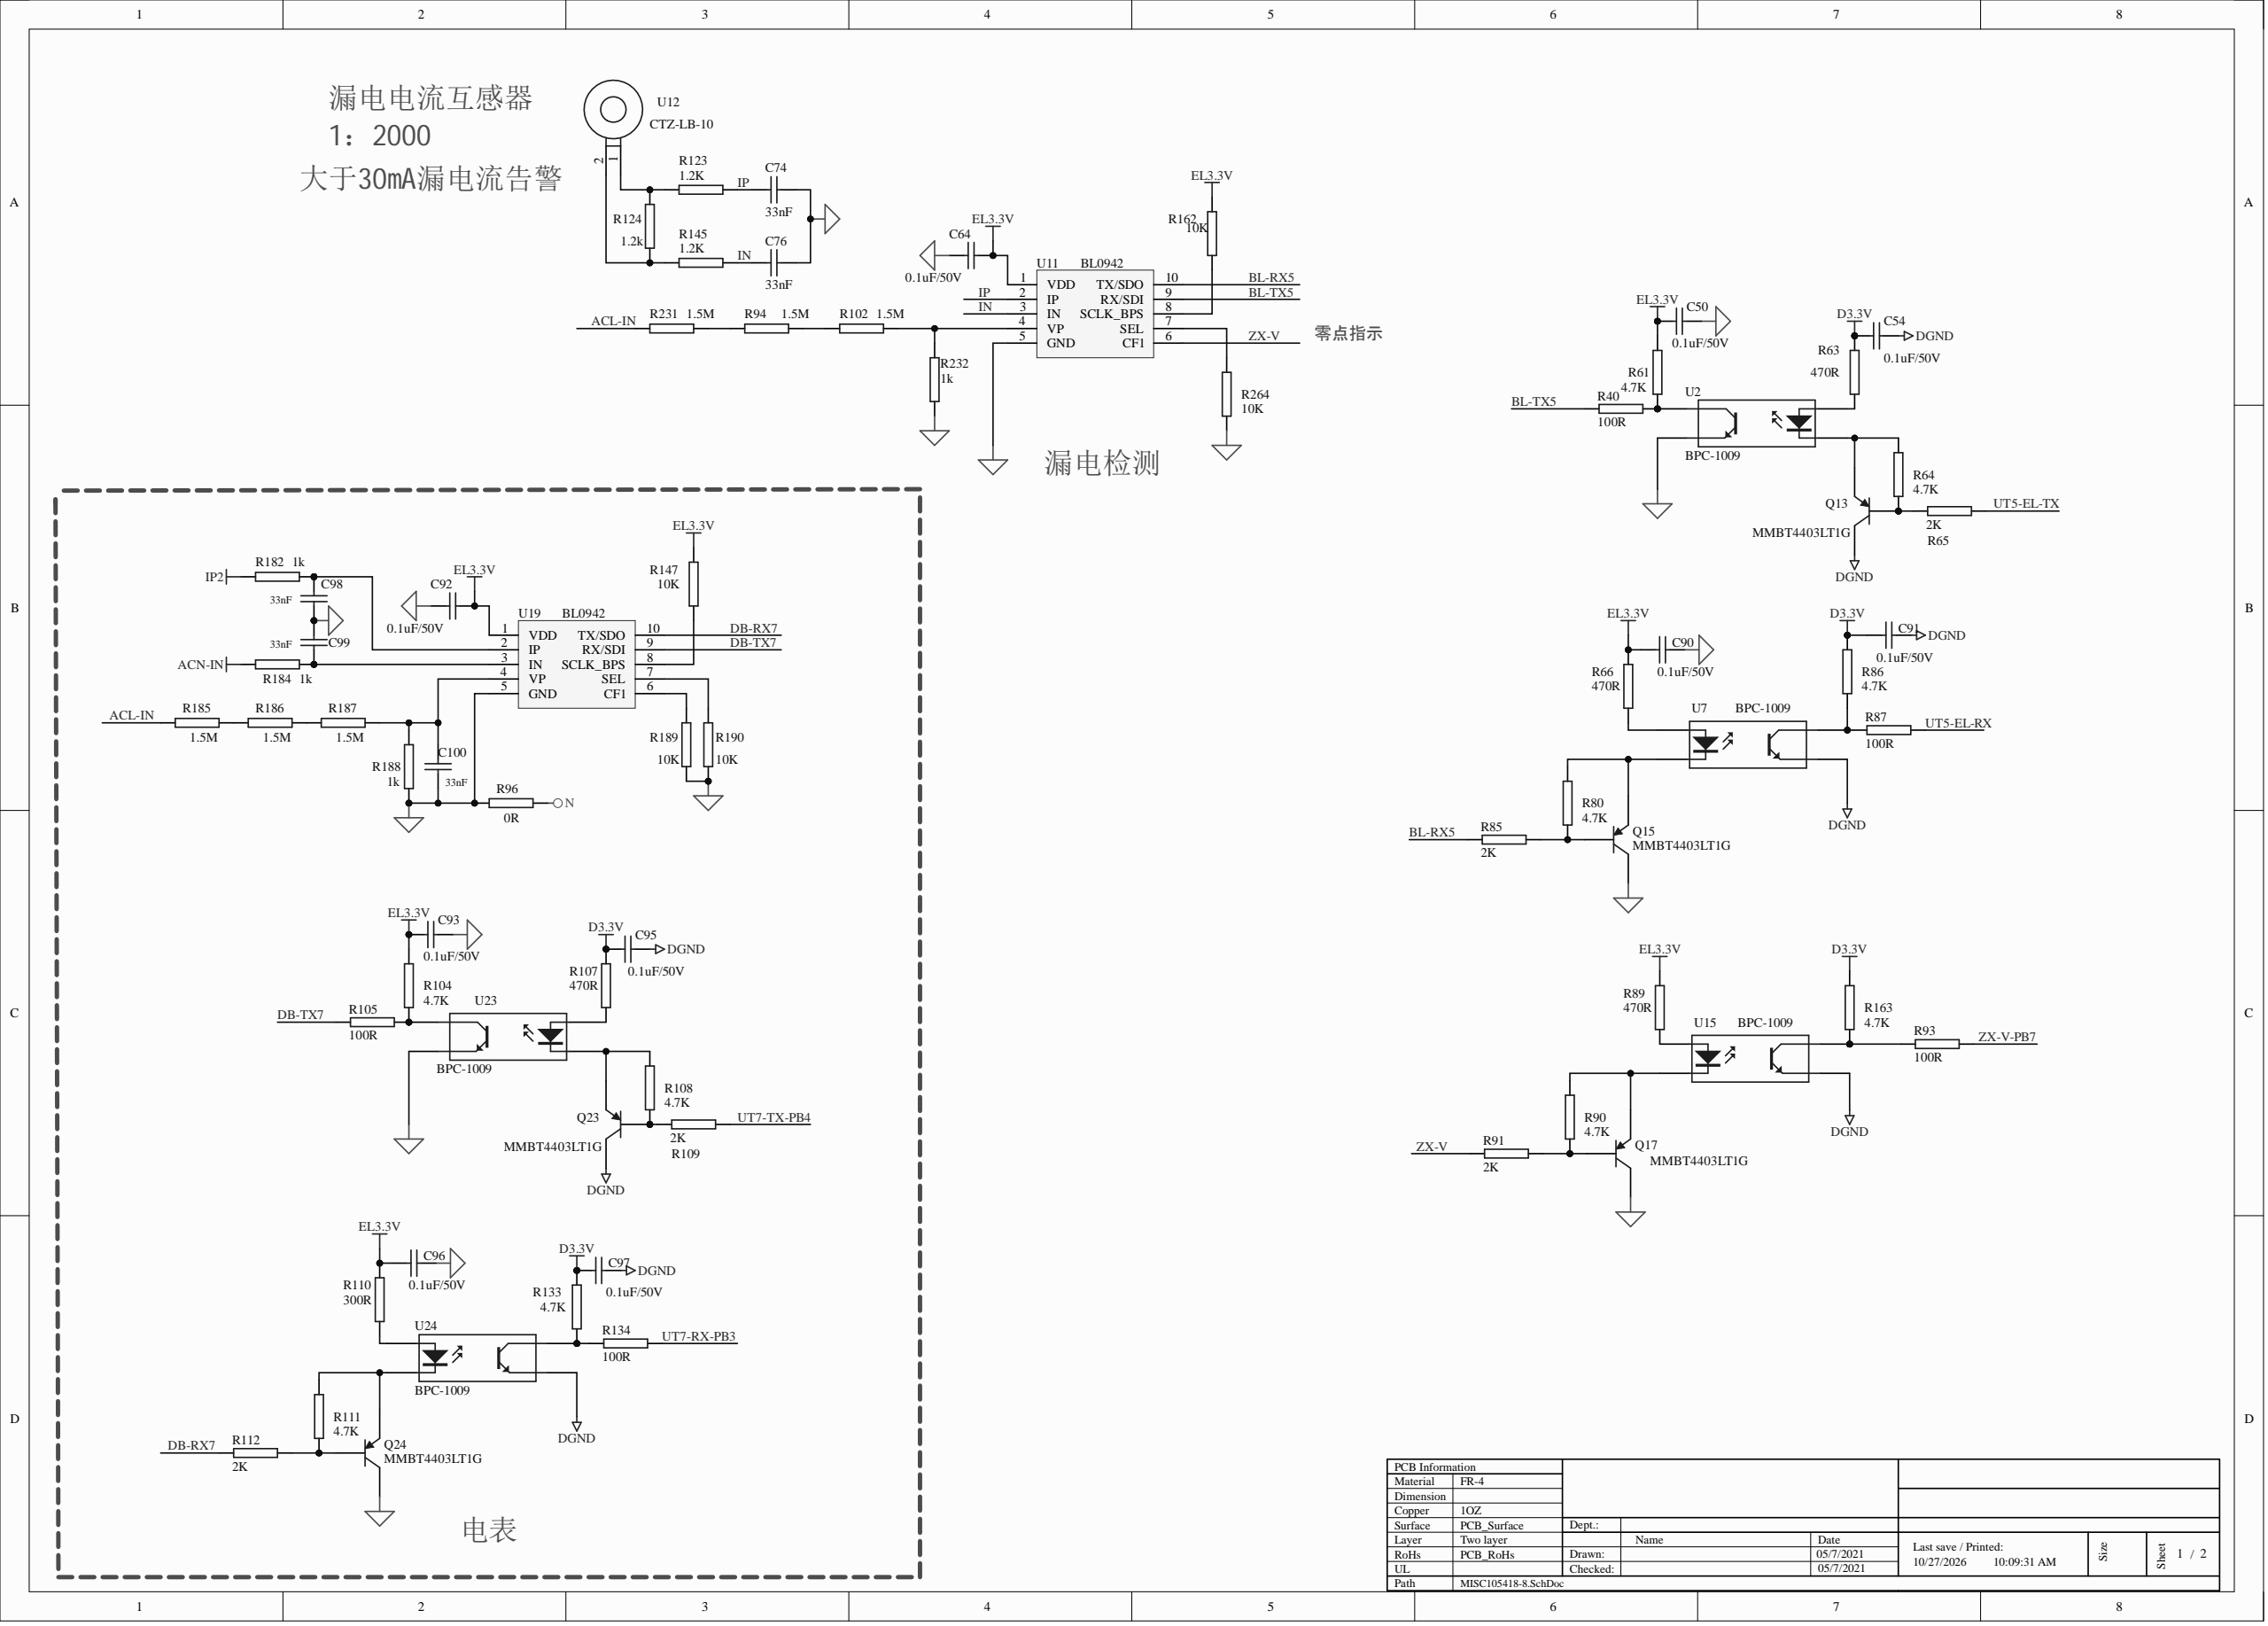Circuit board | Altium Designer | 455 parts | 280 nets | one sheet of the schematic
Parts on this sheet (reference | value | footprint):
C50 | 0.1uF/50V | C0603-T
C54 | 0.1uF/50V | C0603-T
C64 | 0.1uF/50V | C0603-T
C74 | 33nF | C0805-T
C76 | 33nF | C0805-T
C90 | 0.1uF/50V | C0603-T
C91 | 0.1uF/50V | C0603-T
C92 | 0.1uF/50V | C0603-T
C93 | 0.1uF/50V | C0603-T
C95 | 0.1uF/50V | C0603-T
C96 | 0.1uF/50V | C0603-T
C97 | 0.1uF/50V | C0603-T
C98 | 33nF | C0805-T
C99 | 33nF | C0805-T
C100 | 33nF | C0805-T
Q13 | MMBT4403LT1G | SOT-23-T
Q15 | MMBT4403LT1G | SOT-23-T
Q17 | MMBT4403LT1G | SOT-23-T
Q23 | MMBT4403LT1G | SOT-23-T
Q24 | MMBT4403LT1G | SOT-23-T
R40 | 100R | R0603-T
R61 | 4.7K | R0603-T
R63 | 470R | R0805-T
R64 | 4.7K | R0603-T
R65 | 2K | R0603-T
R66 | 470R | R0805-T
R80 | 4.7K | R0603-T
R85 | 2K | R0603-T
R86 | 4.7K | R0603-T
R87 | 100R | R0603-T
R89 | 470R | R0805-T
R90 | 4.7K | R0603-T
R91 | 2K | R0603-T
R93 | 100R | R0603-T
R94 | 1.5M | R0805-T
R96 | 0R | R0805-T
R102 | 1.5M | R0805-T
R104 | 4.7K | R0603-T
R105 | 100R | R0603-T
R107 | 470R | R0805-T
R108 | 4.7K | R0603-T
R109 | 2K | R0603-T
R110 | 300R | R0805-T
R111 | 4.7K | R0603-T
R112 | 2K | R0603-T
R123 | 1.2K | R0805-T
R124 | 1.2K | R0805-T
R133 | 4.7K | R0603-T
R134 | 100R | R0603-T
R145 | 1.2K | R0805-T
R147 | 10K | R0603-T
R162 | 10K | R0603-T
R163 | 4.7K | R0603-T
R182 | 1K | R0805-T
R184 | 1K | R0805-T
R185 | 1.5M | R0805-T
R186 | 1.5M | R0805-T
R187 | 1.5M | R0805-T
R188 | 1K | R0805-T
R189 | 10K | R0603-T
R190 | 10K | R0603-T
R231 | 1.5M | R0805-T
R232 | 1K | R0805-T
R264 | 10K | R0603-T
U2 | BPC-1009 | OPT-SMT(LTV-817S)
U7 | BPC-1009 | OPT-SMT(LTV-817S)
U11 | BL0942 | SO-10-T（脚距1.0mm)
U12 | CTZ-LB-10 | 23012-00041-10  电流互感器
U15 | BPC-1009 | OPT-SMT(LTV-817S)
U19 | BL0942 | SO-10-T（脚距1.0mm)
U23 | BPC-1009 | OPT-SMT(LTV-817S)
U24 | BPC-1009 | OPT-SMT(LTV-817S)
Nets of these parts (net: part-pin ...):
ZX-V-PB7: R93-1
ZX-V: R91-2 U11-6
UT7-TX-PB4: R109-1
UT7-RX-PB3: R134-1
UT5-EL-TX: R65-1
UT5-EL-RX: R87-1
NetR264_2: R264-2 U11-7
NetR190_2: R190-2 U19-7
NetR189_2: R189-2 U19-6
NetR186_1: R186-1 R187-2
NetR185_1: R185-1 R186-2
NetR162_1: R162-1 U11-8
NetR147_1: R147-1 U19-8
NetR133_1: R133-1 R134-2 U24-4
NetR124_2: R124-2 R145-2 U12-2
NetR123_2: R123-2 R124-1 U12-1
NetR110_2: R110-2 U24-1
NetR107_1: R107-1 U23-1
NetR104_1: R104-1 R105-1 U23-4
NetR102_1: R102-1 R232-1 U11-4
NetR94_2: R94-2 R231-1
NetR94_1: R94-1 R102-2
NetR93_2: R93-2 R163-1 U15-4
NetR89_2: R89-2 U15-1
NetR86_1: R86-1 R87-2 U7-4
NetR66_2: R66-2 U7-1
NetR63_1: R63-1 U2-1
NetR40_1: R40-1 R61-1 U2-4
NetQ24_2: Q24-2 R111-2 U24-2
NetQ24_1: Q24-1 R111-1 R112-1
NetQ23_2: Q23-2 R108-2 U23-2
NetQ23_1: Q23-1 R108-1 R109-2
NetQ17_2: Q17-2 R90-2 U15-2
NetQ17_1: Q17-1 R90-1 R91-1
NetQ15_2: Q15-2 R80-2 U7-2
NetQ15_1: Q15-1 R80-1 R85-1
NetQ13_2: Q13-2 R64-2 U2-2
NetQ13_1: Q13-1 R64-1 R65-2
NetC100_1: C100-1 R187-1 R188-1 U19-4
NetC99_2: C99-2 R184-2 U19-3
NetC98_1: C98-1 R182-2 U19-2
N: R96-1
IP2: R182-1
IP: C74-2 R123-1 U11-2
IN: C76-2 R145-1 U11-3
EL3.3V: C50-2 C64-1 C90-2 C92-1 C93-2 C96-2 R61-2 R66-1 R89-1 R104-2 R110-1 R147-2 R162-2 U11-1 U19-1
DBGND: C50-1 C64-2 C74-1 C76-1 C90-1 C92-2 C93-1 C96-1 C98-2 C99-1 C100-2 Q15-3 Q17-3 Q24-3 R96-2 R188-2 R189-1 R190-1 R232-2 R264-1 U2-3 U11-5 U19-5 U23-3
DB-TX7: R105-2 U19-9
DB-RX7: R112-2 U19-10
D3.3V: C54-1 C91-2 C95-1 C97-2 R63-2 R86-2 R107-2 R133-2 R163-2
BL-TX5: R40-2 U11-9
BL-RX5: R85-2 U11-10
ACN-IN: R184-1
ACL-IN: R185-2 R231-2
-: C54-2 C91-1 C95-2 C97-1 Q13-3 Q23-3 U7-3 U15-3 U24-3